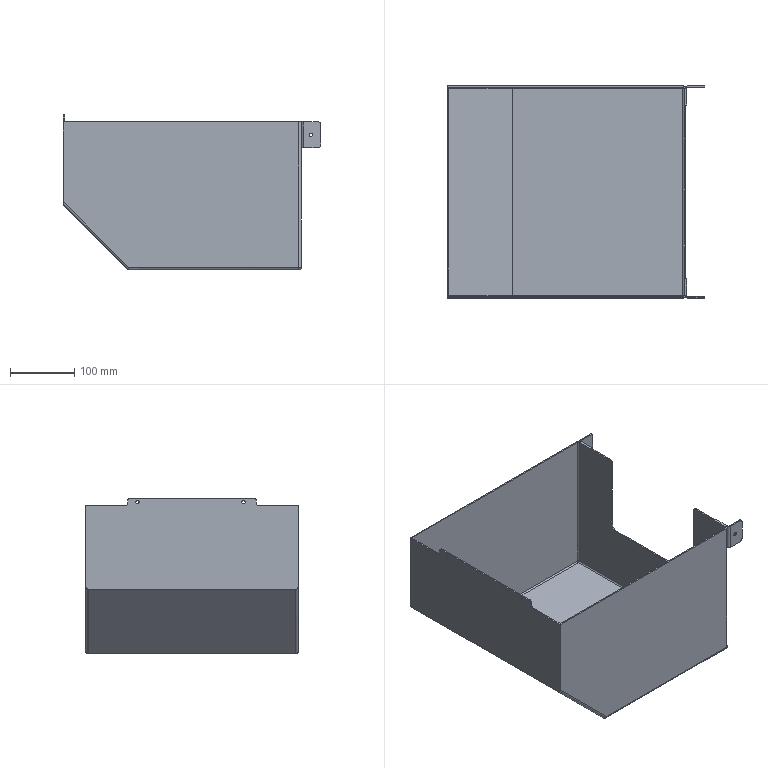Part | NX | features 5003_232_Cover 2 | 1 solid | 70 faces | box 400 x 330 x 242 mm | volume 783768 mm3 | cylinder 34 | plane 32 | sphere 4 | commonest cylinder face diameters 8 x19 4 x9 5.3 x2 5.5 x2 20 x2